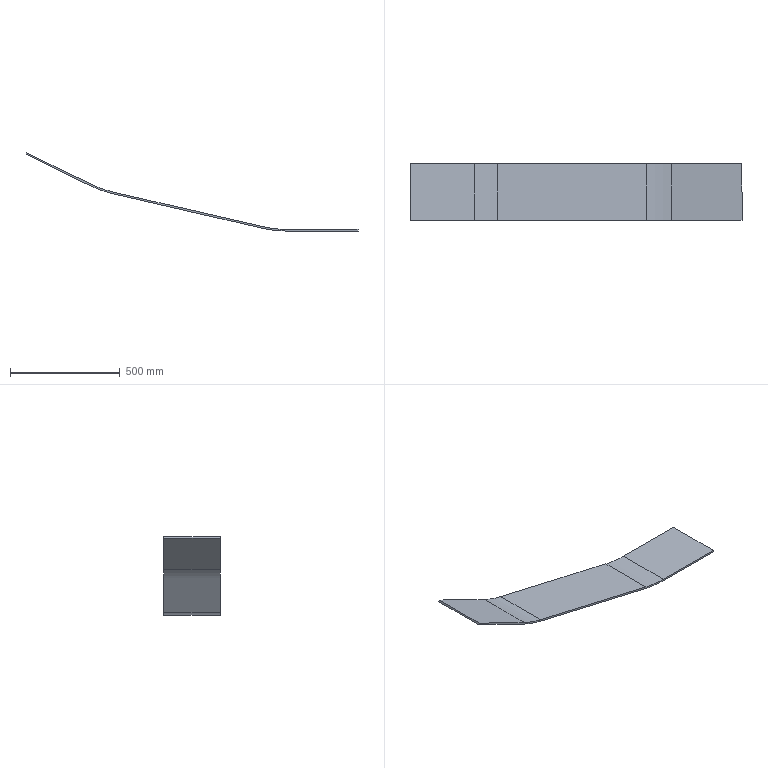Part | SolidWorks | features SM3dBend 2, FlatPattern 1, SMBaseFlange 1, SheetMetal 1 | 1 solid | 22 faces | box 1515 x 258 x 356.966 mm | volume 3243782 mm3 | plane 18 | cylinder 4 | commonest cylinder face diameters 1000 x2 1016 x2
STEP:
#1=CARTESIAN_POINT('',(1134.502,258.,5.02));
#2=VERTEX_POINT('',#1);
#3=CARTESIAN_POINT('',(455.126,258.,161.866));
#4=VERTEX_POINT('',#3);
#5=CARTESIAN_POINT('',(29.154,258.,260.21));
#6=DIRECTION('',(-0.9744,0.,0.225));
#7=VECTOR('',#6,1000.);
#8=LINE('',#5,#7);
#9=EDGE_CURVE('',#2,#4,#8,.T.);
#10=ORIENTED_EDGE('',*,*,#9,.F.);
#11=CARTESIAN_POINT('',(1134.502,0.,5.02));
#12=VERTEX_POINT('',#11);
#13=CARTESIAN_POINT('',(1134.502,258.,5.02));
#14=DIRECTION('',(0.,-1.,0.));
#15=VECTOR('',#14,1000.);
#16=LINE('',#13,#15);
#17=EDGE_CURVE('',#2,#12,#16,.T.);
#18=ORIENTED_EDGE('',*,*,#17,.T.);
#19=CARTESIAN_POINT('',(455.126,0.,161.866));
#20=VERTEX_POINT('',#19);
#21=CARTESIAN_POINT('',(29.154,0.,260.21));
#22=DIRECTION('',(0.9744,0.,-0.225));
#23=VECTOR('',#22,1000.);
#24=LINE('',#21,#23);
#25=EDGE_CURVE('',#20,#12,#24,.T.);
#26=ORIENTED_EDGE('',*,*,#25,.F.);
#27=CARTESIAN_POINT('',(455.126,258.,161.866));
#28=DIRECTION('',(0.,-1.,0.));
#29=VECTOR('',#28,1000.);
#30=LINE('',#27,#29);
#31=EDGE_CURVE('',#4,#20,#30,.T.);
#32=ORIENTED_EDGE('',*,*,#31,.F.);
#33=EDGE_LOOP('',(#10,#18,#26,#32));
#34=FACE_OUTER_BOUND('',#33,.T.);
#35=CARTESIAN_POINT('',(29.154,258.,260.21));
#36=DIRECTION('',(-0.225,0.,-0.9744));
#37=DIRECTION('',(-0.9744,0.,0.225));
#38=AXIS2_PLACEMENT_3D('',#35,#36,#37);
#39=PLANE('',#38);
#40=ADVANCED_FACE('',(#34),#39,.T.);
#41=CARTESIAN_POINT('',(1136.301,258.,12.815));
#42=VERTEX_POINT('',#41);
#43=CARTESIAN_POINT('',(456.926,258.,169.661));
#44=VERTEX_POINT('',#43);
#45=CARTESIAN_POINT('',(30.954,258.,268.005));
#46=DIRECTION('',(-0.9744,0.,0.225));
#47=VECTOR('',#46,1000.);
#48=LINE('',#45,#47);
#49=EDGE_CURVE('',#42,#44,#48,.T.);
#50=ORIENTED_EDGE('',*,*,#49,.F.);
#51=CARTESIAN_POINT('',(1134.502,258.,5.02));
#52=DIRECTION('',(-0.225,0.,-0.9744));
#53=VECTOR('',#52,1000.);
#54=LINE('',#51,#53);
#55=EDGE_CURVE('',#42,#2,#54,.T.);
#56=ORIENTED_EDGE('',*,*,#55,.T.);
#57=ORIENTED_EDGE('',*,*,#9,.T.);
#58=CARTESIAN_POINT('',(455.126,258.,161.866));
#59=DIRECTION('',(-0.225,0.,-0.9744));
#60=VECTOR('',#59,1000.);
#61=LINE('',#58,#60);
#62=EDGE_CURVE('',#44,#4,#61,.T.);
#63=ORIENTED_EDGE('',*,*,#62,.F.);
#64=EDGE_LOOP('',(#50,#56,#57,#63));
#65=FACE_OUTER_BOUND('',#64,.T.);
#66=CARTESIAN_POINT('',(29.154,258.,260.21));
#67=DIRECTION('',(0.,1.,0.));
#68=DIRECTION('',(0.225,0.,0.9744));
#69=AXIS2_PLACEMENT_3D('',#66,#67,#68);
#70=PLANE('',#69);
#71=ADVANCED_FACE('',(#65),#70,.T.);
#72=ORIENTED_EDGE('',*,*,#25,.T.);
#73=CARTESIAN_POINT('',(1136.301,0.,12.815));
#74=VERTEX_POINT('',#73);
#75=CARTESIAN_POINT('',(1134.502,0.,5.02));
#76=DIRECTION('',(0.225,0.,0.9744));
#77=VECTOR('',#76,1000.);
#78=LINE('',#75,#77);
#79=EDGE_CURVE('',#12,#74,#78,.T.);
#80=ORIENTED_EDGE('',*,*,#79,.T.);
#81=CARTESIAN_POINT('',(456.926,0.,169.661));
#82=VERTEX_POINT('',#81);
#83=CARTESIAN_POINT('',(30.954,0.,268.005));
#84=DIRECTION('',(0.9744,0.,-0.225));
#85=VECTOR('',#84,1000.);
#86=LINE('',#83,#85);
#87=EDGE_CURVE('',#82,#74,#86,.T.);
#88=ORIENTED_EDGE('',*,*,#87,.F.);
#89=CARTESIAN_POINT('',(455.126,0.,161.866));
#90=DIRECTION('',(0.225,0.,0.9744));
#91=VECTOR('',#90,1000.);
#92=LINE('',#89,#91);
#93=EDGE_CURVE('',#20,#82,#92,.T.);
#94=ORIENTED_EDGE('',*,*,#93,.F.);
#95=EDGE_LOOP('',(#72,#80,#88,#94));
#96=FACE_OUTER_BOUND('',#95,.T.);
#97=CARTESIAN_POINT('',(29.154,0.,260.21));
#98=DIRECTION('',(0.,-1.,0.));
#99=DIRECTION('',(-0.225,0.,-0.9744));
#100=AXIS2_PLACEMENT_3D('',#97,#98,#99);
#101=PLANE('',#100);
#102=ADVANCED_FACE('',(#96),#101,.T.);
#103=CARTESIAN_POINT('',(350.216,258.,207.449));
#104=VERTEX_POINT('',#103);
#105=CARTESIAN_POINT('',(60.064,258.,348.966));
#106=VERTEX_POINT('',#105);
#107=CARTESIAN_POINT('',(60.064,258.,348.966));
#108=DIRECTION('',(-0.8988,0.,0.4384));
#109=VECTOR('',#108,1000.);
#110=LINE('',#107,#109);
#111=EDGE_CURVE('',#104,#106,#110,.T.);
#112=ORIENTED_EDGE('',*,*,#111,.F.);
#113=CARTESIAN_POINT('',(346.709,258.,200.259));
#114=VERTEX_POINT('',#113);
#115=CARTESIAN_POINT('',(346.709,258.,200.259));
#116=DIRECTION('',(-0.4384,0.,-0.8988));
#117=VECTOR('',#116,1000.);
#118=LINE('',#115,#117);
#119=EDGE_CURVE('',#104,#114,#118,.T.);
#120=ORIENTED_EDGE('',*,*,#119,.T.);
#121=CARTESIAN_POINT('',(56.557,258.,341.775));
#122=VERTEX_POINT('',#121);
#123=CARTESIAN_POINT('',(56.557,258.,341.775));
#124=DIRECTION('',(-0.8988,0.,0.4384));
#125=VECTOR('',#124,1000.);
#126=LINE('',#123,#125);
#127=EDGE_CURVE('',#114,#122,#126,.T.);
#128=ORIENTED_EDGE('',*,*,#127,.T.);
#129=CARTESIAN_POINT('',(56.557,258.,341.775));
#130=DIRECTION('',(0.4384,0.,0.8988));
#131=VECTOR('',#130,1000.);
#132=LINE('',#129,#131);
#133=EDGE_CURVE('',#122,#106,#132,.T.);
#134=ORIENTED_EDGE('',*,*,#133,.T.);
#135=EDGE_LOOP('',(#112,#120,#128,#134));
#136=FACE_OUTER_BOUND('',#135,.T.);
#137=CARTESIAN_POINT('',(56.557,258.,341.775));
#138=DIRECTION('',(0.,1.,0.));
#139=DIRECTION('',(0.4384,0.,0.8988));
#140=AXIS2_PLACEMENT_3D('',#137,#138,#139);
#141=PLANE('',#140);
#142=ADVANCED_FACE('',(#136),#141,.T.);
#143=CARTESIAN_POINT('',(56.557,0.,341.775));
#144=VERTEX_POINT('',#143);
#145=CARTESIAN_POINT('',(346.709,0.,200.259));
#146=VERTEX_POINT('',#145);
#147=CARTESIAN_POINT('',(56.557,0.,341.775));
#148=DIRECTION('',(0.8988,0.,-0.4384));
#149=VECTOR('',#148,1000.);
#150=LINE('',#147,#149);
#151=EDGE_CURVE('',#144,#146,#150,.T.);
#152=ORIENTED_EDGE('',*,*,#151,.T.);
#153=CARTESIAN_POINT('',(350.216,0.,207.449));
#154=VERTEX_POINT('',#153);
#155=CARTESIAN_POINT('',(346.709,0.,200.259));
#156=DIRECTION('',(0.4384,0.,0.8988));
#157=VECTOR('',#156,1000.);
#158=LINE('',#155,#157);
#159=EDGE_CURVE('',#146,#154,#158,.T.);
#160=ORIENTED_EDGE('',*,*,#159,.T.);
#161=CARTESIAN_POINT('',(60.064,0.,348.966));
#162=VERTEX_POINT('',#161);
#163=CARTESIAN_POINT('',(60.064,0.,348.966));
#164=DIRECTION('',(0.8988,0.,-0.4384));
#165=VECTOR('',#164,1000.);
#166=LINE('',#163,#165);
#167=EDGE_CURVE('',#162,#154,#166,.T.);
#168=ORIENTED_EDGE('',*,*,#167,.F.);
#169=CARTESIAN_POINT('',(56.557,0.,341.775));
#170=DIRECTION('',(0.4384,0.,0.8988));
#171=VECTOR('',#170,1000.);
#172=LINE('',#169,#171);
#173=EDGE_CURVE('',#144,#162,#172,.T.);
#174=ORIENTED_EDGE('',*,*,#173,.F.);
#175=EDGE_LOOP('',(#152,#160,#168,#174));
#176=FACE_OUTER_BOUND('',#175,.T.);
#177=CARTESIAN_POINT('',(56.557,0.,341.775));
#178=DIRECTION('',(0.,-1.,0.));
#179=DIRECTION('',(-0.4384,0.,-0.8988));
#180=AXIS2_PLACEMENT_3D('',#177,#178,#179);
#181=PLANE('',#180);
#182=ADVANCED_FACE('',(#176),#181,.T.);
#183=ORIENTED_EDGE('',*,*,#127,.F.);
#184=CARTESIAN_POINT('',(346.709,258.,200.259));
#185=DIRECTION('',(0.,-1.,0.));
#186=VECTOR('',#185,1000.);
#187=LINE('',#184,#186);
#188=EDGE_CURVE('',#114,#146,#187,.T.);
#189=ORIENTED_EDGE('',*,*,#188,.T.);
#190=ORIENTED_EDGE('',*,*,#151,.F.);
#191=CARTESIAN_POINT('',(56.557,0.,341.775));
#192=DIRECTION('',(0.,-1.,0.));
#193=VECTOR('',#192,1000.);
#194=LINE('',#191,#193);
#195=EDGE_CURVE('',#122,#144,#194,.T.);
#196=ORIENTED_EDGE('',*,*,#195,.F.);
#197=EDGE_LOOP('',(#183,#189,#190,#196));
#198=FACE_OUTER_BOUND('',#197,.T.);
#199=CARTESIAN_POINT('',(56.557,258.,341.775));
#200=DIRECTION('',(-0.4384,0.,-0.8988));
#201=DIRECTION('',(-0.8988,0.,0.4384));
#202=AXIS2_PLACEMENT_3D('',#199,#200,#201);
#203=PLANE('',#202);
#204=ADVANCED_FACE('',(#198),#203,.T.);
#205=CARTESIAN_POINT('',(60.064,0.,348.966));
#206=DIRECTION('',(0.,-1.,0.));
#207=VECTOR('',#206,1000.);
#208=LINE('',#205,#207);
#209=EDGE_CURVE('',#106,#162,#208,.T.);
#210=ORIENTED_EDGE('',*,*,#209,.F.);
#211=ORIENTED_EDGE('',*,*,#133,.F.);
#212=ORIENTED_EDGE('',*,*,#195,.T.);
#213=ORIENTED_EDGE('',*,*,#173,.T.);
#214=EDGE_LOOP('',(#210,#211,#212,#213));
#215=FACE_OUTER_BOUND('',#214,.T.);
#216=CARTESIAN_POINT('',(56.557,0.,341.775));
#217=DIRECTION('',(-0.8988,0.,0.4384));
#218=DIRECTION('',(0.4384,0.,0.8988));
#219=AXIS2_PLACEMENT_3D('',#216,#217,#218);
#220=PLANE('',#219);
#221=ADVANCED_FACE('',(#215),#220,.T.);
#222=CARTESIAN_POINT('',(350.216,258.,207.449));
#223=DIRECTION('',(0.,-1.,0.));
#224=VECTOR('',#223,1000.);
#225=LINE('',#222,#224);
#226=EDGE_CURVE('',#104,#154,#225,.T.);
#227=ORIENTED_EDGE('',*,*,#226,.F.);
#228=ORIENTED_EDGE('',*,*,#111,.T.);
#229=ORIENTED_EDGE('',*,*,#209,.T.);
#230=ORIENTED_EDGE('',*,*,#167,.T.);
#231=EDGE_LOOP('',(#227,#228,#229,#230));
#232=FACE_OUTER_BOUND('',#231,.T.);
#233=CARTESIAN_POINT('',(60.064,258.,348.966));
#234=DIRECTION('',(-0.4384,0.,-0.8988));
#235=DIRECTION('',(-0.8988,0.,0.4384));
#236=AXIS2_PLACEMENT_3D('',#233,#234,#235);
#237=PLANE('',#236);
#238=ADVANCED_FACE('',(#232),#237,.F.);
#239=CARTESIAN_POINT('',(1136.301,258.,12.815));
#240=DIRECTION('',(0.,-1.,0.));
#241=VECTOR('',#240,1000.);
#242=LINE('',#239,#241);
#243=EDGE_CURVE('',#42,#74,#242,.T.);
#244=ORIENTED_EDGE('',*,*,#243,.F.);
#245=ORIENTED_EDGE('',*,*,#49,.T.);
#246=CARTESIAN_POINT('',(456.926,258.,169.661));
#247=DIRECTION('',(0.,-1.,0.));
#248=VECTOR('',#247,1000.);
#249=LINE('',#246,#248);
#250=EDGE_CURVE('',#44,#82,#249,.T.);
#251=ORIENTED_EDGE('',*,*,#250,.T.);
#252=ORIENTED_EDGE('',*,*,#87,.T.);
#253=EDGE_LOOP('',(#244,#245,#251,#252));
#254=FACE_OUTER_BOUND('',#253,.T.);
#255=CARTESIAN_POINT('',(30.954,258.,268.005));
#256=DIRECTION('',(-0.225,0.,-0.9744));
#257=DIRECTION('',(-0.9744,0.,0.225));
#258=AXIS2_PLACEMENT_3D('',#255,#256,#257);
#259=PLANE('',#258);
#260=ADVANCED_FACE('',(#254),#259,.F.);
#261=ORIENTED_EDGE('',*,*,#119,.F.);
#262=CARTESIAN_POINT('',(569.401,258.,656.846));
#263=DIRECTION('',(0.,-1.,0.));
#264=DIRECTION('',(-0.9744,0.,0.225));
#265=AXIS2_PLACEMENT_3D('',#262,#263,#264);
#266=CIRCLE('',#265,500.);
#267=EDGE_CURVE('',#104,#44,#266,.T.);
#268=ORIENTED_EDGE('',*,*,#267,.T.);
#269=ORIENTED_EDGE('',*,*,#62,.T.);
#270=CARTESIAN_POINT('',(569.401,258.,656.846));
#271=DIRECTION('',(0.,-1.,0.));
#272=DIRECTION('',(0.225,0.,0.9744));
#273=AXIS2_PLACEMENT_3D('',#270,#271,#272);
#274=CIRCLE('',#273,508.);
#275=EDGE_CURVE('',#114,#4,#274,.T.);
#276=ORIENTED_EDGE('',*,*,#275,.F.);
#277=EDGE_LOOP('',(#261,#268,#269,#276));
#278=FACE_OUTER_BOUND('',#277,.T.);
#279=CARTESIAN_POINT('',(569.401,258.,656.846));
#280=DIRECTION('',(0.,1.,0.));
#281=DIRECTION('',(0.225,0.,0.9744));
#282=AXIS2_PLACEMENT_3D('',#279,#280,#281);
#283=PLANE('',#282);
#284=ADVANCED_FACE('',(#278),#283,.T.);
#285=ORIENTED_EDGE('',*,*,#31,.T.);
#286=CARTESIAN_POINT('',(569.401,0.,656.846));
#287=DIRECTION('',(0.,1.,0.));
#288=DIRECTION('',(0.9744,0.,-0.225));
#289=AXIS2_PLACEMENT_3D('',#286,#287,#288);
#290=CIRCLE('',#289,508.);
#291=EDGE_CURVE('',#20,#146,#290,.T.);
#292=ORIENTED_EDGE('',*,*,#291,.T.);
#293=ORIENTED_EDGE('',*,*,#188,.F.);
#294=ORIENTED_EDGE('',*,*,#275,.T.);
#295=EDGE_LOOP('',(#285,#292,#293,#294));
#296=FACE_OUTER_BOUND('',#295,.T.);
#297=CARTESIAN_POINT('',(569.401,-153.32,656.846));
#298=DIRECTION('',(0.,1.,0.));
#299=DIRECTION('',(-0.9744,0.,0.225));
#300=AXIS2_PLACEMENT_3D('',#297,#298,#299);
#301=CYLINDRICAL_SURFACE('',#300,508.);
#302=ADVANCED_FACE('',(#296),#301,.T.);
#303=CARTESIAN_POINT('',(569.401,0.,656.846));
#304=DIRECTION('',(0.,1.,0.));
#305=DIRECTION('',(-0.9744,0.,0.225));
#306=AXIS2_PLACEMENT_3D('',#303,#304,#305);
#307=CIRCLE('',#306,500.);
#308=EDGE_CURVE('',#82,#154,#307,.T.);
#309=ORIENTED_EDGE('',*,*,#308,.T.);
#310=ORIENTED_EDGE('',*,*,#159,.F.);
#311=ORIENTED_EDGE('',*,*,#291,.F.);
#312=ORIENTED_EDGE('',*,*,#93,.T.);
#313=EDGE_LOOP('',(#309,#310,#311,#312));
#314=FACE_OUTER_BOUND('',#313,.T.);
#315=CARTESIAN_POINT('',(569.401,0.,656.846));
#316=DIRECTION('',(0.,-1.,0.));
#317=DIRECTION('',(0.9744,0.,-0.225));
#318=AXIS2_PLACEMENT_3D('',#315,#316,#317);
#319=PLANE('',#318);
#320=ADVANCED_FACE('',(#314),#319,.T.);
#321=ORIENTED_EDGE('',*,*,#250,.F.);
#322=ORIENTED_EDGE('',*,*,#267,.F.);
#323=ORIENTED_EDGE('',*,*,#226,.T.);
#324=ORIENTED_EDGE('',*,*,#308,.F.);
#325=EDGE_LOOP('',(#321,#322,#323,#324));
#326=FACE_OUTER_BOUND('',#325,.T.);
#327=CARTESIAN_POINT('',(569.401,-153.32,656.846));
#328=DIRECTION('',(0.,1.,0.));
#329=DIRECTION('',(-0.9744,0.,0.225));
#330=AXIS2_PLACEMENT_3D('',#327,#328,#329);
#331=CYLINDRICAL_SURFACE('',#330,500.);
#332=ADVANCED_FACE('',(#326),#331,.F.);
#333=CARTESIAN_POINT('',(1571.6,0.,0.));
#334=VERTEX_POINT('',#333);
#335=CARTESIAN_POINT('',(1571.6,258.,0.));
#336=VERTEX_POINT('',#335);
#337=CARTESIAN_POINT('',(1571.6,0.,0.));
#338=DIRECTION('',(0.,1.,0.));
#339=VECTOR('',#338,1000.);
#340=LINE('',#337,#339);
#341=EDGE_CURVE('',#334,#336,#340,.T.);
#342=ORIENTED_EDGE('',*,*,#341,.F.);
#343=CARTESIAN_POINT('',(1571.6,0.,-8.));
#344=VERTEX_POINT('',#343);
#345=CARTESIAN_POINT('',(1571.6,0.,-8.));
#346=DIRECTION('',(0.,0.,1.));
#347=VECTOR('',#346,1000.);
#348=LINE('',#345,#347);
#349=EDGE_CURVE('',#344,#334,#348,.T.);
#350=ORIENTED_EDGE('',*,*,#349,.F.);
#351=CARTESIAN_POINT('',(1571.6,258.,-8.));
#352=VERTEX_POINT('',#351);
#353=CARTESIAN_POINT('',(1571.6,0.,-8.));
#354=DIRECTION('',(0.,1.,0.));
#355=VECTOR('',#354,1000.);
#356=LINE('',#353,#355);
#357=EDGE_CURVE('',#344,#352,#356,.T.);
#358=ORIENTED_EDGE('',*,*,#357,.T.);
#359=CARTESIAN_POINT('',(1571.6,258.,-8.));
#360=DIRECTION('',(0.,0.,1.));
#361=VECTOR('',#360,1000.);
#362=LINE('',#359,#361);
#363=EDGE_CURVE('',#352,#336,#362,.T.);
#364=ORIENTED_EDGE('',*,*,#363,.T.);
#365=EDGE_LOOP('',(#342,#350,#358,#364));
#366=FACE_OUTER_BOUND('',#365,.T.);
#367=CARTESIAN_POINT('',(1571.6,0.,-8.));
#368=DIRECTION('',(1.,0.,0.));
#369=DIRECTION('',(0.,1.,0.));
#370=AXIS2_PLACEMENT_3D('',#367,#368,#369);
#371=PLANE('',#370);
#372=ADVANCED_FACE('',(#366),#371,.T.);
#373=CARTESIAN_POINT('',(1248.777,258.,-8.));
#374=VERTEX_POINT('',#373);
#375=CARTESIAN_POINT('',(1248.777,0.,-8.));
#376=VERTEX_POINT('',#375);
#377=CARTESIAN_POINT('',(1248.777,258.,-8.));
#378=DIRECTION('',(0.,-1.,0.));
#379=VECTOR('',#378,1000.);
#380=LINE('',#377,#379);
#381=EDGE_CURVE('',#374,#376,#380,.T.);
#382=ORIENTED_EDGE('',*,*,#381,.F.);
#383=CARTESIAN_POINT('',(0.,258.,-8.));
#384=DIRECTION('',(-1.,0.,0.));
#385=VECTOR('',#384,1000.);
#386=LINE('',#383,#385);
#387=EDGE_CURVE('',#352,#374,#386,.T.);
#388=ORIENTED_EDGE('',*,*,#387,.F.);
#389=ORIENTED_EDGE('',*,*,#357,.F.);
#390=CARTESIAN_POINT('',(0.,0.,-8.));
#391=DIRECTION('',(1.,0.,0.));
#392=VECTOR('',#391,1000.);
#393=LINE('',#390,#392);
#394=EDGE_CURVE('',#376,#344,#393,.T.);
#395=ORIENTED_EDGE('',*,*,#394,.F.);
#396=EDGE_LOOP('',(#382,#388,#389,#395));
#397=FACE_OUTER_BOUND('',#396,.T.);
#398=CARTESIAN_POINT('',(0.,258.,-8.));
#399=DIRECTION('',(0.,0.,-1.));
#400=DIRECTION('',(-1.,0.,0.));
#401=AXIS2_PLACEMENT_3D('',#398,#399,#400);
#402=PLANE('',#401);
#403=ADVANCED_FACE('',(#397),#402,.T.);
#404=CARTESIAN_POINT('',(1248.777,258.,0.));
#405=VERTEX_POINT('',#404);
#406=CARTESIAN_POINT('',(1248.777,258.,-8.));
#407=DIRECTION('',(0.,0.,-1.));
#408=VECTOR('',#407,1000.);
#409=LINE('',#406,#408);
#410=EDGE_CURVE('',#405,#374,#409,.T.);
#411=ORIENTED_EDGE('',*,*,#410,.F.);
#412=CARTESIAN_POINT('',(0.,258.,0.));
#413=DIRECTION('',(-1.,0.,0.));
#414=VECTOR('',#413,1000.);
#415=LINE('',#412,#414);
#416=EDGE_CURVE('',#336,#405,#415,.T.);
#417=ORIENTED_EDGE('',*,*,#416,.F.);
#418=ORIENTED_EDGE('',*,*,#363,.F.);
#419=ORIENTED_EDGE('',*,*,#387,.T.);
#420=EDGE_LOOP('',(#411,#417,#418,#419));
#421=FACE_OUTER_BOUND('',#420,.T.);
#422=CARTESIAN_POINT('',(0.,258.,-8.));
#423=DIRECTION('',(0.,1.,0.));
#424=DIRECTION('',(0.,0.,1.));
#425=AXIS2_PLACEMENT_3D('',#422,#423,#424);
#426=PLANE('',#425);
#427=ADVANCED_FACE('',(#421),#426,.T.);
#428=ORIENTED_EDGE('',*,*,#416,.T.);
#429=CARTESIAN_POINT('',(1248.777,0.,0.));
#430=VERTEX_POINT('',#429);
#431=CARTESIAN_POINT('',(1248.777,258.,0.));
#432=DIRECTION('',(0.,-1.,0.));
#433=VECTOR('',#432,1000.);
#434=LINE('',#431,#433);
#435=EDGE_CURVE('',#405,#430,#434,.T.);
#436=ORIENTED_EDGE('',*,*,#435,.T.);
#437=CARTESIAN_POINT('',(0.,0.,0.));
#438=DIRECTION('',(1.,0.,0.));
#439=VECTOR('',#438,1000.);
#440=LINE('',#437,#439);
#441=EDGE_CURVE('',#430,#334,#440,.T.);
#442=ORIENTED_EDGE('',*,*,#441,.T.);
#443=ORIENTED_EDGE('',*,*,#341,.T.);
#444=EDGE_LOOP('',(#428,#436,#442,#443));
#445=FACE_OUTER_BOUND('',#444,.T.);
#446=CARTESIAN_POINT('',(0.,258.,0.));
#447=DIRECTION('',(0.,0.,-1.));
#448=DIRECTION('',(-1.,0.,0.));
#449=AXIS2_PLACEMENT_3D('',#446,#447,#448);
#450=PLANE('',#449);
#451=ADVANCED_FACE('',(#445),#450,.F.);
#452=CARTESIAN_POINT('',(1248.777,0.,-8.));
#453=DIRECTION('',(0.,0.,1.));
#454=VECTOR('',#453,1000.);
#455=LINE('',#452,#454);
#456=EDGE_CURVE('',#376,#430,#455,.T.);
#457=ORIENTED_EDGE('',*,*,#456,.F.);
#458=ORIENTED_EDGE('',*,*,#394,.T.);
#459=ORIENTED_EDGE('',*,*,#349,.T.);
#460=ORIENTED_EDGE('',*,*,#441,.F.);
#461=EDGE_LOOP('',(#457,#458,#459,#460));
#462=FACE_OUTER_BOUND('',#461,.T.);
#463=CARTESIAN_POINT('',(0.,0.,-8.));
#464=DIRECTION('',(0.,-1.,0.));
#465=DIRECTION('',(0.,0.,-1.));
#466=AXIS2_PLACEMENT_3D('',#463,#464,#465);
#467=PLANE('',#466);
#468=ADVANCED_FACE('',(#462),#467,.T.);
#469=ORIENTED_EDGE('',*,*,#55,.F.);
#470=CARTESIAN_POINT('',(1248.777,258.,500.));
#471=DIRECTION('',(0.,-1.,0.));
#472=DIRECTION('',(-1.,0.,0.));
#473=AXIS2_PLACEMENT_3D('',#470,#471,#472);
#474=CIRCLE('',#473,500.);
#475=EDGE_CURVE('',#42,#405,#474,.T.);
#476=ORIENTED_EDGE('',*,*,#475,.T.);
#477=ORIENTED_EDGE('',*,*,#410,.T.);
#478=CARTESIAN_POINT('',(1248.777,258.,500.));
#479=DIRECTION('',(0.,-1.,0.));
#480=DIRECTION('',(0.,0.,1.));
#481=AXIS2_PLACEMENT_3D('',#478,#479,#480);
#482=CIRCLE('',#481,508.);
#483=EDGE_CURVE('',#2,#374,#482,.T.);
#484=ORIENTED_EDGE('',*,*,#483,.F.);
#485=EDGE_LOOP('',(#469,#476,#477,#484));
#486=FACE_OUTER_BOUND('',#485,.T.);
#487=CARTESIAN_POINT('',(1248.777,258.,500.));
#488=DIRECTION('',(0.,1.,0.));
#489=DIRECTION('',(0.,0.,1.));
#490=AXIS2_PLACEMENT_3D('',#487,#488,#489);
#491=PLANE('',#490);
#492=ADVANCED_FACE('',(#486),#491,.T.);
#493=ORIENTED_EDGE('',*,*,#381,.T.);
#494=CARTESIAN_POINT('',(1248.777,0.,500.));
#495=DIRECTION('',(0.,1.,0.));
#496=DIRECTION('',(1.,0.,0.));
#497=AXIS2_PLACEMENT_3D('',#494,#495,#496);
#498=CIRCLE('',#497,508.);
#499=EDGE_CURVE('',#376,#12,#498,.T.);
#500=ORIENTED_EDGE('',*,*,#499,.T.);
#501=ORIENTED_EDGE('',*,*,#17,.F.);
#502=ORIENTED_EDGE('',*,*,#483,.T.);
#503=EDGE_LOOP('',(#493,#500,#501,#502));
#504=FACE_OUTER_BOUND('',#503,.T.);
#505=CARTESIAN_POINT('',(1248.777,-153.32,500.));
#506=DIRECTION('',(0.,1.,0.));
#507=DIRECTION('',(-1.,0.,0.));
#508=AXIS2_PLACEMENT_3D('',#505,#506,#507);
#509=CYLINDRICAL_SURFACE('',#508,508.);
#510=ADVANCED_FACE('',(#504),#509,.T.);
#511=CARTESIAN_POINT('',(1248.777,0.,500.));
#512=DIRECTION('',(0.,1.,0.));
#513=DIRECTION('',(-1.,0.,0.));
#514=AXIS2_PLACEMENT_3D('',#511,#512,#513);
#515=CIRCLE('',#514,500.);
#516=EDGE_CURVE('',#430,#74,#515,.T.);
#517=ORIENTED_EDGE('',*,*,#516,.T.);
#518=ORIENTED_EDGE('',*,*,#79,.F.);
#519=ORIENTED_EDGE('',*,*,#499,.F.);
#520=ORIENTED_EDGE('',*,*,#456,.T.);
#521=EDGE_LOOP('',(#517,#518,#519,#520));
#522=FACE_OUTER_BOUND('',#521,.T.);
#523=CARTESIAN_POINT('',(1248.777,0.,500.));
#524=DIRECTION('',(0.,-1.,0.));
#525=DIRECTION('',(1.,0.,0.));
#526=AXIS2_PLACEMENT_3D('',#523,#524,#525);
#527=PLANE('',#526);
#528=ADVANCED_FACE('',(#522),#527,.T.);
#529=ORIENTED_EDGE('',*,*,#435,.F.);
#530=ORIENTED_EDGE('',*,*,#475,.F.);
#531=ORIENTED_EDGE('',*,*,#243,.T.);
#532=ORIENTED_EDGE('',*,*,#516,.F.);
#533=EDGE_LOOP('',(#529,#530,#531,#532));
#534=FACE_OUTER_BOUND('',#533,.T.);
#535=CARTESIAN_POINT('',(1248.777,-153.32,500.));
#536=DIRECTION('',(0.,1.,0.));
#537=DIRECTION('',(-1.,0.,0.));
#538=AXIS2_PLACEMENT_3D('',#535,#536,#537);
#539=CYLINDRICAL_SURFACE('',#538,500.);
#540=ADVANCED_FACE('',(#534),#539,.F.);
#541=CLOSED_SHELL('',(#40,#71,#102,#142,#182,#204,#221,#238,#260,#284,#302,#320,#332,#372,#403,#427,#451,#468,#492,#510,#528,#540));
#542=MANIFOLD_SOLID_BREP('',#541);
#543=CARTESIAN_POINT('',(0.,0.,0.));
#544=DIRECTION('',(0.,0.,1.));
#545=DIRECTION('',(1.,0.,0.));
#546=AXIS2_PLACEMENT_3D('',#543,#544,#545);
#547=(LENGTH_UNIT()NAMED_UNIT(*)SI_UNIT(.MILLI.,.METRE.));
#548=UNCERTAINTY_MEASURE_WITH_UNIT(LENGTH_MEASURE(0.00001),#547,'','');
#549=(NAMED_UNIT(*)PLANE_ANGLE_UNIT()SI_UNIT($,.RADIAN.));
#550=(NAMED_UNIT(*)SI_UNIT($,.STERADIAN.)SOLID_ANGLE_UNIT());
#551=(GEOMETRIC_REPRESENTATION_CONTEXT(3)GLOBAL_UNCERTAINTY_ASSIGNED_CONTEXT((#548))GLOBAL_UNIT_ASSIGNED_CONTEXT((#547,#549,#550))REPRESENTATION_CONTEXT('',''));
#552=ADVANCED_BREP_SHAPE_REPRESENTATION('',(#542,#546),#551);